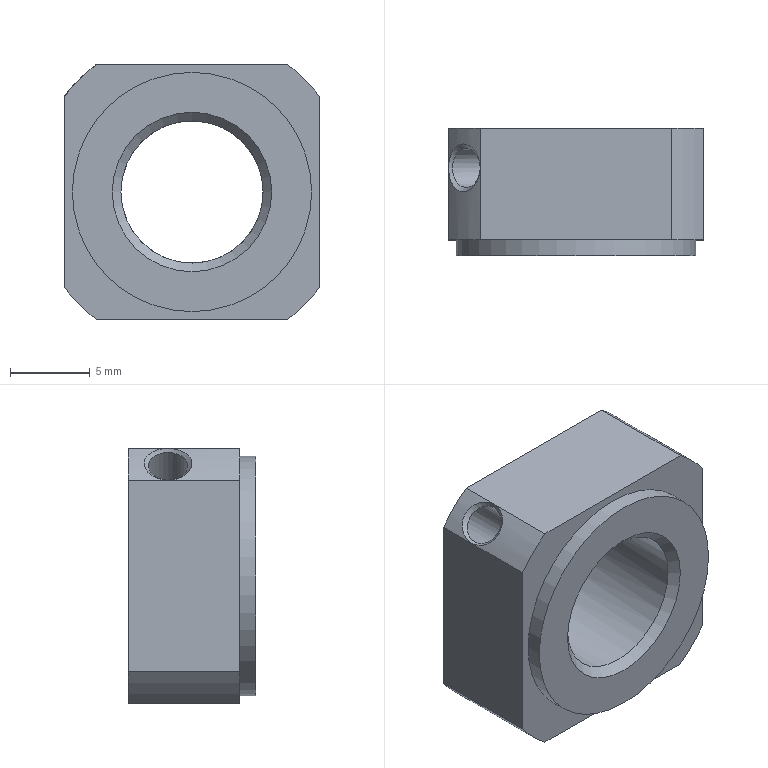Part | STEP file | ROTATION MC_NEW VER-0610_488 | 1 solid | 17 faces | box 16 x 8 x 16 mm | volume 1383 mm3 | cylinder 7 | plane 7 | cone 3 | commonest cylinder face diameters 20 x4 2.459 x1 8.917 x1 15 x1
STEP:
#1=CARTESIAN_POINT('',(-238.48,689.468,-78.342));
#2=VERTEX_POINT('',#1);
#3=CARTESIAN_POINT('',(-240.218,689.468,-80.081));
#4=VERTEX_POINT('',#3);
#5=CARTESIAN_POINT('',(-239.349,689.468,-79.211));
#6=DIRECTION('',(0.7071,0.,-0.7071));
#7=DIRECTION('',(-0.7071,0.,-0.7071));
#8=AXIS2_PLACEMENT_3D('',#5,#6,#7);
#9=CIRCLE('',#8,1.23);
#10=EDGE_CURVE('',#2,#4,#9,.T.);
#11=ORIENTED_EDGE('',*,*,#10,.F.);
#12=CARTESIAN_POINT('',(-239.349,689.468,-79.211));
#13=DIRECTION('',(0.7071,0.,-0.7071));
#14=DIRECTION('',(-0.7071,0.,-0.7071));
#15=AXIS2_PLACEMENT_3D('',#12,#13,#14);
#16=CIRCLE('',#15,1.23);
#17=EDGE_CURVE('',#4,#2,#16,.T.);
#18=ORIENTED_EDGE('',*,*,#17,.F.);
#19=CARTESIAN_POINT('',(-236.369,689.468,-83.93));
#20=VERTEX_POINT('',#19);
#21=CARTESIAN_POINT('',(-233.339,689.468,-86.961));
#22=DIRECTION('',(0.7071,0.,-0.7071));
#23=VECTOR('',#22,1.23);
#24=LINE('',#21,#23);
#25=EDGE_CURVE('',#4,#20,#24,.T.);
#26=ORIENTED_EDGE('',*,*,#25,.T.);
#27=CARTESIAN_POINT('',(-236.369,689.468,-83.93));
#28=CARTESIAN_POINT('',(-236.369,689.313,-83.93));
#29=CARTESIAN_POINT('',(-236.354,689.148,-83.902));
#30=CARTESIAN_POINT('',(-236.288,688.845,-83.789));
#31=CARTESIAN_POINT('',(-236.238,688.708,-83.706));
#32=CARTESIAN_POINT('',(-236.115,688.49,-83.522));
#33=CARTESIAN_POINT('',(-236.033,688.396,-83.408));
#34=CARTESIAN_POINT('',(-235.842,688.27,-83.171));
#35=CARTESIAN_POINT('',(-235.732,688.239,-83.048));
#36=CARTESIAN_POINT('',(-235.512,688.239,-82.829));
#37=CARTESIAN_POINT('',(-235.389,688.27,-82.718));
#38=CARTESIAN_POINT('',(-235.152,688.396,-82.527));
#39=CARTESIAN_POINT('',(-235.039,688.49,-82.446));
#40=CARTESIAN_POINT('',(-234.855,688.708,-82.323));
#41=CARTESIAN_POINT('',(-234.771,688.845,-82.272));
#42=CARTESIAN_POINT('',(-234.659,689.148,-82.207));
#43=CARTESIAN_POINT('',(-234.63,689.313,-82.192));
#44=CARTESIAN_POINT('',(-234.63,689.624,-82.192));
#45=CARTESIAN_POINT('',(-234.659,689.789,-82.207));
#46=CARTESIAN_POINT('',(-234.771,690.091,-82.272));
#47=CARTESIAN_POINT('',(-234.855,690.229,-82.323));
#48=CARTESIAN_POINT('',(-235.039,690.446,-82.446));
#49=CARTESIAN_POINT('',(-235.152,690.541,-82.527));
#50=CARTESIAN_POINT('',(-235.389,690.667,-82.718));
#51=CARTESIAN_POINT('',(-235.512,690.698,-82.829));
#52=CARTESIAN_POINT('',(-235.732,690.698,-83.048));
#53=CARTESIAN_POINT('',(-235.842,690.667,-83.171));
#54=CARTESIAN_POINT('',(-236.033,690.541,-83.408));
#55=CARTESIAN_POINT('',(-236.115,690.446,-83.522));
#56=CARTESIAN_POINT('',(-236.238,690.229,-83.706));
#57=CARTESIAN_POINT('',(-236.288,690.091,-83.789));
#58=CARTESIAN_POINT('',(-236.354,689.789,-83.902));
#59=CARTESIAN_POINT('',(-236.369,689.624,-83.93));
#60=CARTESIAN_POINT('',(-236.369,689.468,-83.93));
#61=B_SPLINE_CURVE_WITH_KNOTS('',3,(#27,#28,#29,#30,#31,#32,#33,#34,#35,#36,#37,#38,#39,#40,#41,#42,#43,#44,#45,#46,#47,#48,#49,#50,#51,#52,#53,#54,#55,#56,#57,#58,#59,#60),.UNSPECIFIED.,.T.,.F.,(4,2,2,2,2,2,2,2,2,2,2,2,2,2,2,2,4),(-0.7452,-0.6986,-0.652,-0.6055,-0.5589,-0.5123,-0.4658,-0.4192,-0.3726,-0.326,-0.2794,-0.2329,-0.1863,-0.1397,-0.09316,-0.04658,0.),.UNSPECIFIED.);
#62=EDGE_CURVE('',#20,#20,#61,.T.);
#63=ORIENTED_EDGE('',*,*,#62,.F.);
#64=ORIENTED_EDGE('',*,*,#25,.F.);
#65=EDGE_LOOP('',(#11,#18,#26,#63,#64));
#66=FACE_OUTER_BOUND('',#65,.T.);
#67=CARTESIAN_POINT('',(-232.469,689.468,-86.091));
#68=DIRECTION('',(0.7071,0.,-0.7071));
#69=DIRECTION('',(0.7071,0.,0.7071));
#70=AXIS2_PLACEMENT_3D('',#67,#68,#69);
#71=CYLINDRICAL_SURFACE('',#70,1.23);
#72=ADVANCED_FACE('',(#66),#71,.F.);
#73=ORIENTED_EDGE('',*,*,#10,.T.);
#74=ORIENTED_EDGE('',*,*,#17,.T.);
#75=CARTESIAN_POINT('',(-238.48,689.468,-78.099));
#76=VERTEX_POINT('',#75);
#77=CARTESIAN_POINT('',(-238.48,689.468,-77.96));
#78=DIRECTION('',(-0.000000001,0.,1.));
#79=VECTOR('',#78,1.5);
#80=LINE('',#77,#79);
#81=EDGE_CURVE('',#2,#76,#80,.T.);
#82=ORIENTED_EDGE('',*,*,#81,.T.);
#83=CARTESIAN_POINT('',(-238.48,689.468,-78.099));
#84=CARTESIAN_POINT('',(-238.48,689.649,-78.099));
#85=CARTESIAN_POINT('',(-238.506,689.844,-78.119));
#86=CARTESIAN_POINT('',(-238.614,690.205,-78.202));
#87=CARTESIAN_POINT('',(-238.696,690.372,-78.265));
#88=CARTESIAN_POINT('',(-238.885,690.643,-78.42));
#89=CARTESIAN_POINT('',(-239.006,690.764,-78.522));
#90=CARTESIAN_POINT('',(-239.269,690.927,-78.757));
#91=CARTESIAN_POINT('',(-239.41,690.968,-78.89));
#92=CARTESIAN_POINT('',(-239.67,690.968,-79.15));
#93=CARTESIAN_POINT('',(-239.804,690.927,-79.292));
#94=CARTESIAN_POINT('',(-240.039,690.764,-79.554));
#95=CARTESIAN_POINT('',(-240.141,690.643,-79.676));
#96=CARTESIAN_POINT('',(-240.295,690.372,-79.865));
#97=CARTESIAN_POINT('',(-240.359,690.205,-79.946));
#98=CARTESIAN_POINT('',(-240.442,689.844,-80.054));
#99=CARTESIAN_POINT('',(-240.461,689.649,-80.081));
#100=CARTESIAN_POINT('',(-240.461,689.287,-80.081));
#101=CARTESIAN_POINT('',(-240.442,689.093,-80.054));
#102=CARTESIAN_POINT('',(-240.359,688.732,-79.946));
#103=CARTESIAN_POINT('',(-240.295,688.565,-79.865));
#104=CARTESIAN_POINT('',(-240.141,688.294,-79.676));
#105=CARTESIAN_POINT('',(-240.039,688.172,-79.554));
#106=CARTESIAN_POINT('',(-239.804,688.01,-79.292));
#107=CARTESIAN_POINT('',(-239.67,687.968,-79.15));
#108=CARTESIAN_POINT('',(-239.41,687.968,-78.89));
#109=CARTESIAN_POINT('',(-239.269,688.01,-78.757));
#110=CARTESIAN_POINT('',(-239.006,688.172,-78.522));
#111=CARTESIAN_POINT('',(-238.885,688.294,-78.42));
#112=CARTESIAN_POINT('',(-238.696,688.565,-78.265));
#113=CARTESIAN_POINT('',(-238.614,688.732,-78.202));
#114=CARTESIAN_POINT('',(-238.506,689.093,-78.119));
#115=CARTESIAN_POINT('',(-238.48,689.287,-78.099));
#116=CARTESIAN_POINT('',(-238.48,689.468,-78.099));
#117=B_SPLINE_CURVE_WITH_KNOTS('',3,(#83,#84,#85,#86,#87,#88,#89,#90,#91,#92,#93,#94,#95,#96,#97,#98,#99,#100,#101,#102,#103,#104,#105,#106,#107,#108,#109,#110,#111,#112,#113,#114,#115,#116),.UNSPECIFIED.,.T.,.F.,(4,2,2,2,2,2,2,2,2,2,2,2,2,2,2,2,4),(-0.8757,-0.8214,-0.7671,-0.7119,-0.6568,-0.6016,-0.5464,-0.4921,-0.4378,-0.3835,-0.3292,-0.2741,-0.2189,-0.1638,-0.1086,-0.0543,0.),.UNSPECIFIED.);
#118=EDGE_CURVE('',#76,#76,#117,.T.);
#119=ORIENTED_EDGE('',*,*,#118,.T.);
#120=ORIENTED_EDGE('',*,*,#81,.F.);
#121=EDGE_LOOP('',(#73,#74,#82,#119,#120));
#122=FACE_OUTER_BOUND('',#121,.T.);
#123=CARTESIAN_POINT('',(-239.54,689.468,-79.02));
#124=DIRECTION('',(-0.7071,0.,0.7071));
#125=DIRECTION('',(-0.7071,0.,-0.7071));
#126=AXIS2_PLACEMENT_3D('',#123,#124,#125);
#127=CONICAL_SURFACE('',#126,1.5,0.7854);
#128=ADVANCED_FACE('',(#122),#127,.F.);
#129=CARTESIAN_POINT('',(-236.928,691.427,-86.091));
#130=VERTEX_POINT('',#129);
#131=CARTESIAN_POINT('',(-232.469,691.427,-86.091));
#132=DIRECTION('',(0.,1.,0.));
#133=DIRECTION('',(-1.,0.,0.));
#134=AXIS2_PLACEMENT_3D('',#131,#132,#133);
#135=CIRCLE('',#134,4.458);
#136=EDGE_CURVE('',#130,#130,#135,.T.);
#137=ORIENTED_EDGE('',*,*,#136,.F.);
#138=CARTESIAN_POINT('',(-237.469,691.968,-86.091));
#139=VERTEX_POINT('',#138);
#140=CARTESIAN_POINT('',(-236.928,691.427,-86.091));
#141=DIRECTION('',(-0.7071,0.7071,0.));
#142=VECTOR('',#141,4.458);
#143=LINE('',#140,#142);
#144=EDGE_CURVE('',#130,#139,#143,.T.);
#145=ORIENTED_EDGE('',*,*,#144,.T.);
#146=CARTESIAN_POINT('',(-232.469,691.968,-86.091));
#147=DIRECTION('',(0.,1.,0.));
#148=DIRECTION('',(-1.,0.,0.));
#149=AXIS2_PLACEMENT_3D('',#146,#147,#148);
#150=CIRCLE('',#149,5.);
#151=EDGE_CURVE('',#139,#139,#150,.T.);
#152=ORIENTED_EDGE('',*,*,#151,.T.);
#153=ORIENTED_EDGE('',*,*,#144,.F.);
#154=EDGE_LOOP('',(#137,#145,#152,#153));
#155=FACE_OUTER_BOUND('',#154,.T.);
#156=CARTESIAN_POINT('',(-232.469,691.427,-86.091));
#157=DIRECTION('',(0.,1.,0.));
#158=DIRECTION('',(1.,0.,0.));
#159=AXIS2_PLACEMENT_3D('',#156,#157,#158);
#160=CONICAL_SURFACE('',#159,4.458,0.7854);
#161=ADVANCED_FACE('',(#155),#160,.F.);
#162=CARTESIAN_POINT('',(-236.928,684.51,-86.091));
#163=VERTEX_POINT('',#162);
#164=CARTESIAN_POINT('',(-228.011,684.51,-86.091));
#165=VERTEX_POINT('',#164);
#166=CARTESIAN_POINT('',(-232.469,684.51,-86.091));
#167=DIRECTION('',(0.,1.,0.));
#168=DIRECTION('',(-1.,0.,0.));
#169=AXIS2_PLACEMENT_3D('',#166,#167,#168);
#170=CIRCLE('',#169,4.458);
#171=EDGE_CURVE('',#163,#165,#170,.T.);
#172=ORIENTED_EDGE('',*,*,#171,.T.);
#173=CARTESIAN_POINT('',(-227.469,683.968,-86.091));
#174=VERTEX_POINT('',#173);
#175=CARTESIAN_POINT('',(-227.469,683.968,-86.091));
#176=DIRECTION('',(0.7071,-0.7071,0.));
#177=VECTOR('',#176,5.);
#178=LINE('',#175,#177);
#179=EDGE_CURVE('',#165,#174,#178,.T.);
#180=ORIENTED_EDGE('',*,*,#179,.T.);
#181=CARTESIAN_POINT('',(-237.469,683.968,-86.091));
#182=VERTEX_POINT('',#181);
#183=CARTESIAN_POINT('',(-232.469,683.968,-86.091));
#184=DIRECTION('',(0.,1.,0.));
#185=DIRECTION('',(-1.,0.,0.));
#186=AXIS2_PLACEMENT_3D('',#183,#184,#185);
#187=CIRCLE('',#186,5.);
#188=EDGE_CURVE('',#182,#174,#187,.T.);
#189=ORIENTED_EDGE('',*,*,#188,.F.);
#190=CARTESIAN_POINT('',(-232.469,683.968,-86.091));
#191=DIRECTION('',(0.,1.,0.));
#192=DIRECTION('',(-1.,0.,0.));
#193=AXIS2_PLACEMENT_3D('',#190,#191,#192);
#194=CIRCLE('',#193,5.);
#195=EDGE_CURVE('',#174,#182,#194,.T.);
#196=ORIENTED_EDGE('',*,*,#195,.F.);
#197=ORIENTED_EDGE('',*,*,#179,.F.);
#198=CARTESIAN_POINT('',(-232.469,684.51,-86.091));
#199=DIRECTION('',(0.,1.,0.));
#200=DIRECTION('',(-1.,0.,0.));
#201=AXIS2_PLACEMENT_3D('',#198,#199,#200);
#202=CIRCLE('',#201,4.458);
#203=EDGE_CURVE('',#165,#163,#202,.T.);
#204=ORIENTED_EDGE('',*,*,#203,.T.);
#205=EDGE_LOOP('',(#172,#180,#189,#196,#197,#204));
#206=FACE_OUTER_BOUND('',#205,.T.);
#207=CARTESIAN_POINT('',(-232.469,683.968,-86.091));
#208=DIRECTION('',(0.,-1.,0.));
#209=DIRECTION('',(-1.,0.,0.));
#210=AXIS2_PLACEMENT_3D('',#207,#208,#209);
#211=CONICAL_SURFACE('',#210,5.,0.7854);
#212=ADVANCED_FACE('',(#206),#211,.F.);
#213=CARTESIAN_POINT('',(-239.969,684.968,-86.091));
#214=VERTEX_POINT('',#213);
#215=CARTESIAN_POINT('',(-232.469,684.968,-86.091));
#216=DIRECTION('',(0.,-1.,0.));
#217=DIRECTION('',(-1.,0.,0.));
#218=AXIS2_PLACEMENT_3D('',#215,#216,#217);
#219=CIRCLE('',#218,7.5);
#220=EDGE_CURVE('',#214,#214,#219,.T.);
#221=ORIENTED_EDGE('',*,*,#220,.T.);
#222=CARTESIAN_POINT('',(-239.969,683.968,-86.091));
#223=VERTEX_POINT('',#222);
#224=CARTESIAN_POINT('',(-239.969,684.968,-86.091));
#225=DIRECTION('',(0.,-1.,0.));
#226=VECTOR('',#225,7.5);
#227=LINE('',#224,#226);
#228=EDGE_CURVE('',#214,#223,#227,.T.);
#229=ORIENTED_EDGE('',*,*,#228,.T.);
#230=CARTESIAN_POINT('',(-232.469,683.968,-86.091));
#231=DIRECTION('',(0.,1.,0.));
#232=DIRECTION('',(-1.,0.,0.));
#233=AXIS2_PLACEMENT_3D('',#230,#231,#232);
#234=CIRCLE('',#233,7.5);
#235=EDGE_CURVE('',#223,#223,#234,.T.);
#236=ORIENTED_EDGE('',*,*,#235,.T.);
#237=ORIENTED_EDGE('',*,*,#228,.F.);
#238=EDGE_LOOP('',(#221,#229,#236,#237));
#239=FACE_OUTER_BOUND('',#238,.T.);
#240=CARTESIAN_POINT('',(-232.469,684.968,-86.091));
#241=DIRECTION('',(0.,1.,0.));
#242=DIRECTION('',(1.,0.,0.));
#243=AXIS2_PLACEMENT_3D('',#240,#241,#242);
#244=CYLINDRICAL_SURFACE('',#243,7.5);
#245=ADVANCED_FACE('',(#239),#244,.T.);
#246=ORIENTED_EDGE('',*,*,#235,.F.);
#247=EDGE_LOOP('',(#246));
#248=FACE_OUTER_BOUND('',#247,.T.);
#249=ORIENTED_EDGE('',*,*,#188,.T.);
#250=ORIENTED_EDGE('',*,*,#195,.T.);
#251=EDGE_LOOP('',(#249,#250));
#252=FACE_BOUND('',#251,.T.);
#253=CARTESIAN_POINT('',(-232.469,683.968,-86.091));
#254=DIRECTION('',(0.,1.,0.));
#255=DIRECTION('',(0.,0.,1.));
#256=AXIS2_PLACEMENT_3D('',#253,#254,#255);
#257=PLANE('',#256);
#258=ADVANCED_FACE('',(#248,#252),#257,.F.);
#259=CARTESIAN_POINT('',(-226.469,684.968,-78.091));
#260=VERTEX_POINT('',#259);
#261=CARTESIAN_POINT('',(-224.469,684.968,-80.091));
#262=VERTEX_POINT('',#261);
#263=CARTESIAN_POINT('',(-232.469,684.968,-86.091));
#264=DIRECTION('',(0.,1.,0.));
#265=DIRECTION('',(-1.,0.,0.));
#266=AXIS2_PLACEMENT_3D('',#263,#264,#265);
#267=CIRCLE('',#266,10.);
#268=EDGE_CURVE('',#260,#262,#267,.T.);
#269=ORIENTED_EDGE('',*,*,#268,.F.);
#270=CARTESIAN_POINT('',(-238.469,684.968,-78.091));
#271=VERTEX_POINT('',#270);
#272=CARTESIAN_POINT('',(-238.469,684.968,-78.091));
#273=DIRECTION('',(1.,0.,0.));
#274=VECTOR('',#273,12.);
#275=LINE('',#272,#274);
#276=EDGE_CURVE('',#271,#260,#275,.T.);
#277=ORIENTED_EDGE('',*,*,#276,.F.);
#278=CARTESIAN_POINT('',(-240.469,684.968,-80.091));
#279=VERTEX_POINT('',#278);
#280=CARTESIAN_POINT('',(-232.469,684.968,-86.091));
#281=DIRECTION('',(0.,1.,0.));
#282=DIRECTION('',(-1.,0.,0.));
#283=AXIS2_PLACEMENT_3D('',#280,#281,#282);
#284=CIRCLE('',#283,10.);
#285=EDGE_CURVE('',#279,#271,#284,.T.);
#286=ORIENTED_EDGE('',*,*,#285,.F.);
#287=CARTESIAN_POINT('',(-240.469,684.968,-92.091));
#288=VERTEX_POINT('',#287);
#289=CARTESIAN_POINT('',(-240.469,684.968,-92.091));
#290=DIRECTION('',(0.,0.,1.));
#291=VECTOR('',#290,12.);
#292=LINE('',#289,#291);
#293=EDGE_CURVE('',#288,#279,#292,.T.);
#294=ORIENTED_EDGE('',*,*,#293,.F.);
#295=CARTESIAN_POINT('',(-238.469,684.968,-94.091));
#296=VERTEX_POINT('',#295);
#297=CARTESIAN_POINT('',(-232.469,684.968,-86.091));
#298=DIRECTION('',(0.,1.,0.));
#299=DIRECTION('',(-1.,0.,0.));
#300=AXIS2_PLACEMENT_3D('',#297,#298,#299);
#301=CIRCLE('',#300,10.);
#302=EDGE_CURVE('',#296,#288,#301,.T.);
#303=ORIENTED_EDGE('',*,*,#302,.F.);
#304=CARTESIAN_POINT('',(-226.469,684.968,-94.091));
#305=VERTEX_POINT('',#304);
#306=CARTESIAN_POINT('',(-226.469,684.968,-94.091));
#307=DIRECTION('',(-1.,0.,0.));
#308=VECTOR('',#307,12.);
#309=LINE('',#306,#308);
#310=EDGE_CURVE('',#305,#296,#309,.T.);
#311=ORIENTED_EDGE('',*,*,#310,.F.);
#312=CARTESIAN_POINT('',(-224.469,684.968,-92.091));
#313=VERTEX_POINT('',#312);
#314=CARTESIAN_POINT('',(-232.469,684.968,-86.091));
#315=DIRECTION('',(0.,1.,0.));
#316=DIRECTION('',(-1.,0.,0.));
#317=AXIS2_PLACEMENT_3D('',#314,#315,#316);
#318=CIRCLE('',#317,10.);
#319=EDGE_CURVE('',#313,#305,#318,.T.);
#320=ORIENTED_EDGE('',*,*,#319,.F.);
#321=CARTESIAN_POINT('',(-224.469,684.968,-80.091));
#322=DIRECTION('',(0.,0.,-1.));
#323=VECTOR('',#322,12.);
#324=LINE('',#321,#323);
#325=EDGE_CURVE('',#262,#313,#324,.T.);
#326=ORIENTED_EDGE('',*,*,#325,.F.);
#327=EDGE_LOOP('',(#269,#277,#286,#294,#303,#311,#320,#326));
#328=FACE_OUTER_BOUND('',#327,.T.);
#329=ORIENTED_EDGE('',*,*,#220,.F.);
#330=EDGE_LOOP('',(#329));
#331=FACE_BOUND('',#330,.T.);
#332=CARTESIAN_POINT('',(-232.469,684.968,-86.091));
#333=DIRECTION('',(0.,1.,0.));
#334=DIRECTION('',(0.,0.,1.));
#335=AXIS2_PLACEMENT_3D('',#332,#333,#334);
#336=PLANE('',#335);
#337=ADVANCED_FACE('',(#328,#331),#336,.F.);
#338=CARTESIAN_POINT('',(-226.469,691.968,-78.091));
#339=VERTEX_POINT('',#338);
#340=CARTESIAN_POINT('',(-224.469,691.968,-80.091));
#341=VERTEX_POINT('',#340);
#342=CARTESIAN_POINT('',(-232.469,691.968,-86.091));
#343=DIRECTION('',(0.,1.,0.));
#344=DIRECTION('',(-1.,0.,0.));
#345=AXIS2_PLACEMENT_3D('',#342,#343,#344);
#346=CIRCLE('',#345,10.);
#347=EDGE_CURVE('',#339,#341,#346,.T.);
#348=ORIENTED_EDGE('',*,*,#347,.T.);
#349=CARTESIAN_POINT('',(-224.469,691.968,-92.091));
#350=VERTEX_POINT('',#349);
#351=CARTESIAN_POINT('',(-224.469,691.968,-80.091));
#352=DIRECTION('',(0.,0.,-1.));
#353=VECTOR('',#352,12.);
#354=LINE('',#351,#353);
#355=EDGE_CURVE('',#341,#350,#354,.T.);
#356=ORIENTED_EDGE('',*,*,#355,.T.);
#357=CARTESIAN_POINT('',(-226.469,691.968,-94.091));
#358=VERTEX_POINT('',#357);
#359=CARTESIAN_POINT('',(-232.469,691.968,-86.091));
#360=DIRECTION('',(0.,1.,0.));
#361=DIRECTION('',(-1.,0.,0.));
#362=AXIS2_PLACEMENT_3D('',#359,#360,#361);
#363=CIRCLE('',#362,10.);
#364=EDGE_CURVE('',#350,#358,#363,.T.);
#365=ORIENTED_EDGE('',*,*,#364,.T.);
#366=CARTESIAN_POINT('',(-238.469,691.968,-94.091));
#367=VERTEX_POINT('',#366);
#368=CARTESIAN_POINT('',(-226.469,691.968,-94.091));
#369=DIRECTION('',(-1.,0.,0.));
#370=VECTOR('',#369,12.);
#371=LINE('',#368,#370);
#372=EDGE_CURVE('',#358,#367,#371,.T.);
#373=ORIENTED_EDGE('',*,*,#372,.T.);
#374=CARTESIAN_POINT('',(-240.469,691.968,-92.091));
#375=VERTEX_POINT('',#374);
#376=CARTESIAN_POINT('',(-232.469,691.968,-86.091));
#377=DIRECTION('',(0.,1.,0.));
#378=DIRECTION('',(-1.,0.,0.));
#379=AXIS2_PLACEMENT_3D('',#376,#377,#378);
#380=CIRCLE('',#379,10.);
#381=EDGE_CURVE('',#367,#375,#380,.T.);
#382=ORIENTED_EDGE('',*,*,#381,.T.);
#383=CARTESIAN_POINT('',(-240.469,691.968,-80.091));
#384=VERTEX_POINT('',#383);
#385=CARTESIAN_POINT('',(-240.469,691.968,-92.091));
#386=DIRECTION('',(0.,0.,1.));
#387=VECTOR('',#386,12.);
#388=LINE('',#385,#387);
#389=EDGE_CURVE('',#375,#384,#388,.T.);
#390=ORIENTED_EDGE('',*,*,#389,.T.);
#391=CARTESIAN_POINT('',(-238.469,691.968,-78.091));
#392=VERTEX_POINT('',#391);
#393=CARTESIAN_POINT('',(-232.469,691.968,-86.091));
#394=DIRECTION('',(0.,1.,0.));
#395=DIRECTION('',(-1.,0.,0.));
#396=AXIS2_PLACEMENT_3D('',#393,#394,#395);
#397=CIRCLE('',#396,10.);
#398=EDGE_CURVE('',#384,#392,#397,.T.);
#399=ORIENTED_EDGE('',*,*,#398,.T.);
#400=CARTESIAN_POINT('',(-238.469,691.968,-78.091));
#401=DIRECTION('',(1.,0.,0.));
#402=VECTOR('',#401,12.);
#403=LINE('',#400,#402);
#404=EDGE_CURVE('',#392,#339,#403,.T.);
#405=ORIENTED_EDGE('',*,*,#404,.T.);
#406=EDGE_LOOP('',(#348,#356,#365,#373,#382,#390,#399,#405));
#407=FACE_OUTER_BOUND('',#406,.T.);
#408=ORIENTED_EDGE('',*,*,#151,.F.);
#409=EDGE_LOOP('',(#408));
#410=FACE_BOUND('',#409,.T.);
#411=CARTESIAN_POINT('',(-232.469,691.968,-86.091));
#412=DIRECTION('',(0.,1.,0.));
#413=DIRECTION('',(0.,0.,1.));
#414=AXIS2_PLACEMENT_3D('',#411,#412,#413);
#415=PLANE('',#414);
#416=ADVANCED_FACE('',(#407,#410),#415,.T.);
#417=ORIENTED_EDGE('',*,*,#276,.T.);
#418=CARTESIAN_POINT('',(-226.469,691.968,-78.091));
#419=DIRECTION('',(0.,-1.,0.));
#420=VECTOR('',#419,7.);
#421=LINE('',#418,#420);
#422=EDGE_CURVE('',#339,#260,#421,.T.);
#423=ORIENTED_EDGE('',*,*,#422,.F.);
#424=ORIENTED_EDGE('',*,*,#404,.F.);
#425=CARTESIAN_POINT('',(-238.469,691.968,-78.091));
#426=DIRECTION('',(0.,-1.,0.));
#427=VECTOR('',#426,7.);
#428=LINE('',#425,#427);
#429=EDGE_CURVE('',#392,#271,#428,.T.);
#430=ORIENTED_EDGE('',*,*,#429,.T.);
#431=EDGE_LOOP('',(#417,#423,#424,#430));
#432=FACE_OUTER_BOUND('',#431,.T.);
#433=CARTESIAN_POINT('',(-238.469,691.968,-78.091));
#434=DIRECTION('',(0.,0.,-1.));
#435=DIRECTION('',(-1.,0.,0.));
#436=AXIS2_PLACEMENT_3D('',#433,#434,#435);
#437=PLANE('',#436);
#438=ADVANCED_FACE('',(#432),#437,.F.);
#439=ORIENTED_EDGE('',*,*,#293,.T.);
#440=CARTESIAN_POINT('',(-240.469,691.968,-80.091));
#441=DIRECTION('',(0.,-1.,0.));
#442=VECTOR('',#441,7.);
#443=LINE('',#440,#442);
#444=EDGE_CURVE('',#384,#279,#443,.T.);
#445=ORIENTED_EDGE('',*,*,#444,.F.);
#446=ORIENTED_EDGE('',*,*,#389,.F.);
#447=CARTESIAN_POINT('',(-240.469,691.968,-92.091));
#448=DIRECTION('',(0.,-1.,0.));
#449=VECTOR('',#448,7.);
#450=LINE('',#447,#449);
#451=EDGE_CURVE('',#375,#288,#450,.T.);
#452=ORIENTED_EDGE('',*,*,#451,.T.);
#453=EDGE_LOOP('',(#439,#445,#446,#452));
#454=FACE_OUTER_BOUND('',#453,.T.);
#455=CARTESIAN_POINT('',(-240.469,691.968,-92.091));
#456=DIRECTION('',(1.,0.,0.));
#457=DIRECTION('',(0.,0.,-1.));
#458=AXIS2_PLACEMENT_3D('',#455,#456,#457);
#459=PLANE('',#458);
#460=ADVANCED_FACE('',(#454),#459,.F.);
#461=ORIENTED_EDGE('',*,*,#302,.T.);
#462=ORIENTED_EDGE('',*,*,#451,.F.);
#463=ORIENTED_EDGE('',*,*,#381,.F.);
#464=CARTESIAN_POINT('',(-238.469,691.968,-94.091));
#465=DIRECTION('',(0.,-1.,0.));
#466=VECTOR('',#465,7.);
#467=LINE('',#464,#466);
#468=EDGE_CURVE('',#367,#296,#467,.T.);
#469=ORIENTED_EDGE('',*,*,#468,.T.);
#470=EDGE_LOOP('',(#461,#462,#463,#469));
#471=FACE_OUTER_BOUND('',#470,.T.);
#472=CARTESIAN_POINT('',(-232.469,691.968,-86.091));
#473=DIRECTION('',(0.,-1.,0.));
#474=DIRECTION('',(-1.,0.,0.));
#475=AXIS2_PLACEMENT_3D('',#472,#473,#474);
#476=CYLINDRICAL_SURFACE('',#475,10.);
#477=ADVANCED_FACE('',(#471),#476,.T.);
#478=ORIENTED_EDGE('',*,*,#310,.T.);
#479=ORIENTED_EDGE('',*,*,#468,.F.);
#480=ORIENTED_EDGE('',*,*,#372,.F.);
#481=CARTESIAN_POINT('',(-226.469,691.968,-94.091));
#482=DIRECTION('',(0.,-1.,0.));
#483=VECTOR('',#482,7.);
#484=LINE('',#481,#483);
#485=EDGE_CURVE('',#358,#305,#484,.T.);
#486=ORIENTED_EDGE('',*,*,#485,.T.);
#487=EDGE_LOOP('',(#478,#479,#480,#486));
#488=FACE_OUTER_BOUND('',#487,.T.);
#489=CARTESIAN_POINT('',(-226.469,691.968,-94.091));
#490=DIRECTION('',(0.,0.,1.));
#491=DIRECTION('',(1.,0.,0.));
#492=AXIS2_PLACEMENT_3D('',#489,#490,#491);
#493=PLANE('',#492);
#494=ADVANCED_FACE('',(#488),#493,.F.);
#495=ORIENTED_EDGE('',*,*,#319,.T.);
#496=ORIENTED_EDGE('',*,*,#485,.F.);
#497=ORIENTED_EDGE('',*,*,#364,.F.);
#498=CARTESIAN_POINT('',(-224.469,691.968,-92.091));
#499=DIRECTION('',(0.,-1.,0.));
#500=VECTOR('',#499,7.);
#501=LINE('',#498,#500);
#502=EDGE_CURVE('',#350,#313,#501,.T.);
#503=ORIENTED_EDGE('',*,*,#502,.T.);
#504=EDGE_LOOP('',(#495,#496,#497,#503));
#505=FACE_OUTER_BOUND('',#504,.T.);
#506=CARTESIAN_POINT('',(-232.469,691.968,-86.091));
#507=DIRECTION('',(0.,-1.,0.));
#508=DIRECTION('',(-1.,0.,0.));
#509=AXIS2_PLACEMENT_3D('',#506,#507,#508);
#510=CYLINDRICAL_SURFACE('',#509,10.);
#511=ADVANCED_FACE('',(#505),#510,.T.);
#512=ORIENTED_EDGE('',*,*,#325,.T.);
#513=ORIENTED_EDGE('',*,*,#502,.F.);
#514=ORIENTED_EDGE('',*,*,#355,.F.);
#515=CARTESIAN_POINT('',(-224.469,691.968,-80.091));
#516=DIRECTION('',(0.,-1.,0.));
#517=VECTOR('',#516,7.);
#518=LINE('',#515,#517);
#519=EDGE_CURVE('',#341,#262,#518,.T.);
#520=ORIENTED_EDGE('',*,*,#519,.T.);
#521=EDGE_LOOP('',(#512,#513,#514,#520));
#522=FACE_OUTER_BOUND('',#521,.T.);
#523=CARTESIAN_POINT('',(-224.469,691.968,-80.091));
#524=DIRECTION('',(-1.,0.,0.));
#525=DIRECTION('',(0.,0.,1.));
#526=AXIS2_PLACEMENT_3D('',#523,#524,#525);
#527=PLANE('',#526);
#528=ADVANCED_FACE('',(#522),#527,.F.);
#529=ORIENTED_EDGE('',*,*,#268,.T.);
#530=ORIENTED_EDGE('',*,*,#519,.F.);
#531=ORIENTED_EDGE('',*,*,#347,.F.);
#532=ORIENTED_EDGE('',*,*,#422,.T.);
#533=EDGE_LOOP('',(#529,#530,#531,#532));
#534=FACE_OUTER_BOUND('',#533,.T.);
#535=CARTESIAN_POINT('',(-232.469,691.968,-86.091));
#536=DIRECTION('',(0.,-1.,0.));
#537=DIRECTION('',(-1.,0.,0.));
#538=AXIS2_PLACEMENT_3D('',#535,#536,#537);
#539=CYLINDRICAL_SURFACE('',#538,10.);
#540=ADVANCED_FACE('',(#534),#539,.T.);
#541=ORIENTED_EDGE('',*,*,#171,.F.);
#542=CARTESIAN_POINT('',(-236.928,691.968,-86.091));
#543=DIRECTION('',(0.,1.,0.));
#544=VECTOR('',#543,4.458);
#545=LINE('',#542,#544);
#546=EDGE_CURVE('',#163,#130,#545,.T.);
#547=ORIENTED_EDGE('',*,*,#546,.T.);
#548=ORIENTED_EDGE('',*,*,#136,.T.);
#549=ORIENTED_EDGE('',*,*,#546,.F.);
#550=ORIENTED_EDGE('',*,*,#203,.F.);
#551=EDGE_LOOP('',(#541,#547,#548,#549,#550));
#552=FACE_OUTER_BOUND('',#551,.T.);
#553=ORIENTED_EDGE('',*,*,#62,.T.);
#554=EDGE_LOOP('',(#553));
#555=FACE_BOUND('',#554,.T.);
#556=CARTESIAN_POINT('',(-232.469,691.968,-86.091));
#557=DIRECTION('',(0.,1.,0.));
#558=DIRECTION('',(1.,0.,0.));
#559=AXIS2_PLACEMENT_3D('',#556,#557,#558);
#560=CYLINDRICAL_SURFACE('',#559,4.458);
#561=ADVANCED_FACE('',(#552,#555),#560,.F.);
#562=ORIENTED_EDGE('',*,*,#285,.T.);
#563=ORIENTED_EDGE('',*,*,#429,.F.);
#564=ORIENTED_EDGE('',*,*,#398,.F.);
#565=ORIENTED_EDGE('',*,*,#444,.T.);
#566=EDGE_LOOP('',(#562,#563,#564,#565));
#567=FACE_OUTER_BOUND('',#566,.T.);
#568=ORIENTED_EDGE('',*,*,#118,.F.);
#569=EDGE_LOOP('',(#568));
#570=FACE_BOUND('',#569,.T.);
#571=CARTESIAN_POINT('',(-232.469,691.968,-86.091));
#572=DIRECTION('',(0.,-1.,0.));
#573=DIRECTION('',(-1.,0.,0.));
#574=AXIS2_PLACEMENT_3D('',#571,#572,#573);
#575=CYLINDRICAL_SURFACE('',#574,10.);
#576=ADVANCED_FACE('',(#567,#570),#575,.T.);
#577=CLOSED_SHELL('',(#72,#128,#161,#212,#245,#258,#337,#416,#438,#460,#477,#494,#511,#528,#540,#561,#576));
#578=MANIFOLD_SOLID_BREP('',#577);
#579=(LENGTH_UNIT()NAMED_UNIT(*)SI_UNIT(.MILLI.,.METRE.));
#580=UNCERTAINTY_MEASURE_WITH_UNIT(LENGTH_MEASURE(0.01),#579,'','');
#581=(NAMED_UNIT(*)PLANE_ANGLE_UNIT()SI_UNIT($,.RADIAN.));
#582=(NAMED_UNIT(*)SI_UNIT($,.STERADIAN.)SOLID_ANGLE_UNIT());
#583=(GEOMETRIC_REPRESENTATION_CONTEXT(3)GLOBAL_UNCERTAINTY_ASSIGNED_CONTEXT((#580))GLOBAL_UNIT_ASSIGNED_CONTEXT((#579,#581,#582))REPRESENTATION_CONTEXT('',''));
#584=ADVANCED_BREP_SHAPE_REPRESENTATION('',(#578),#583);